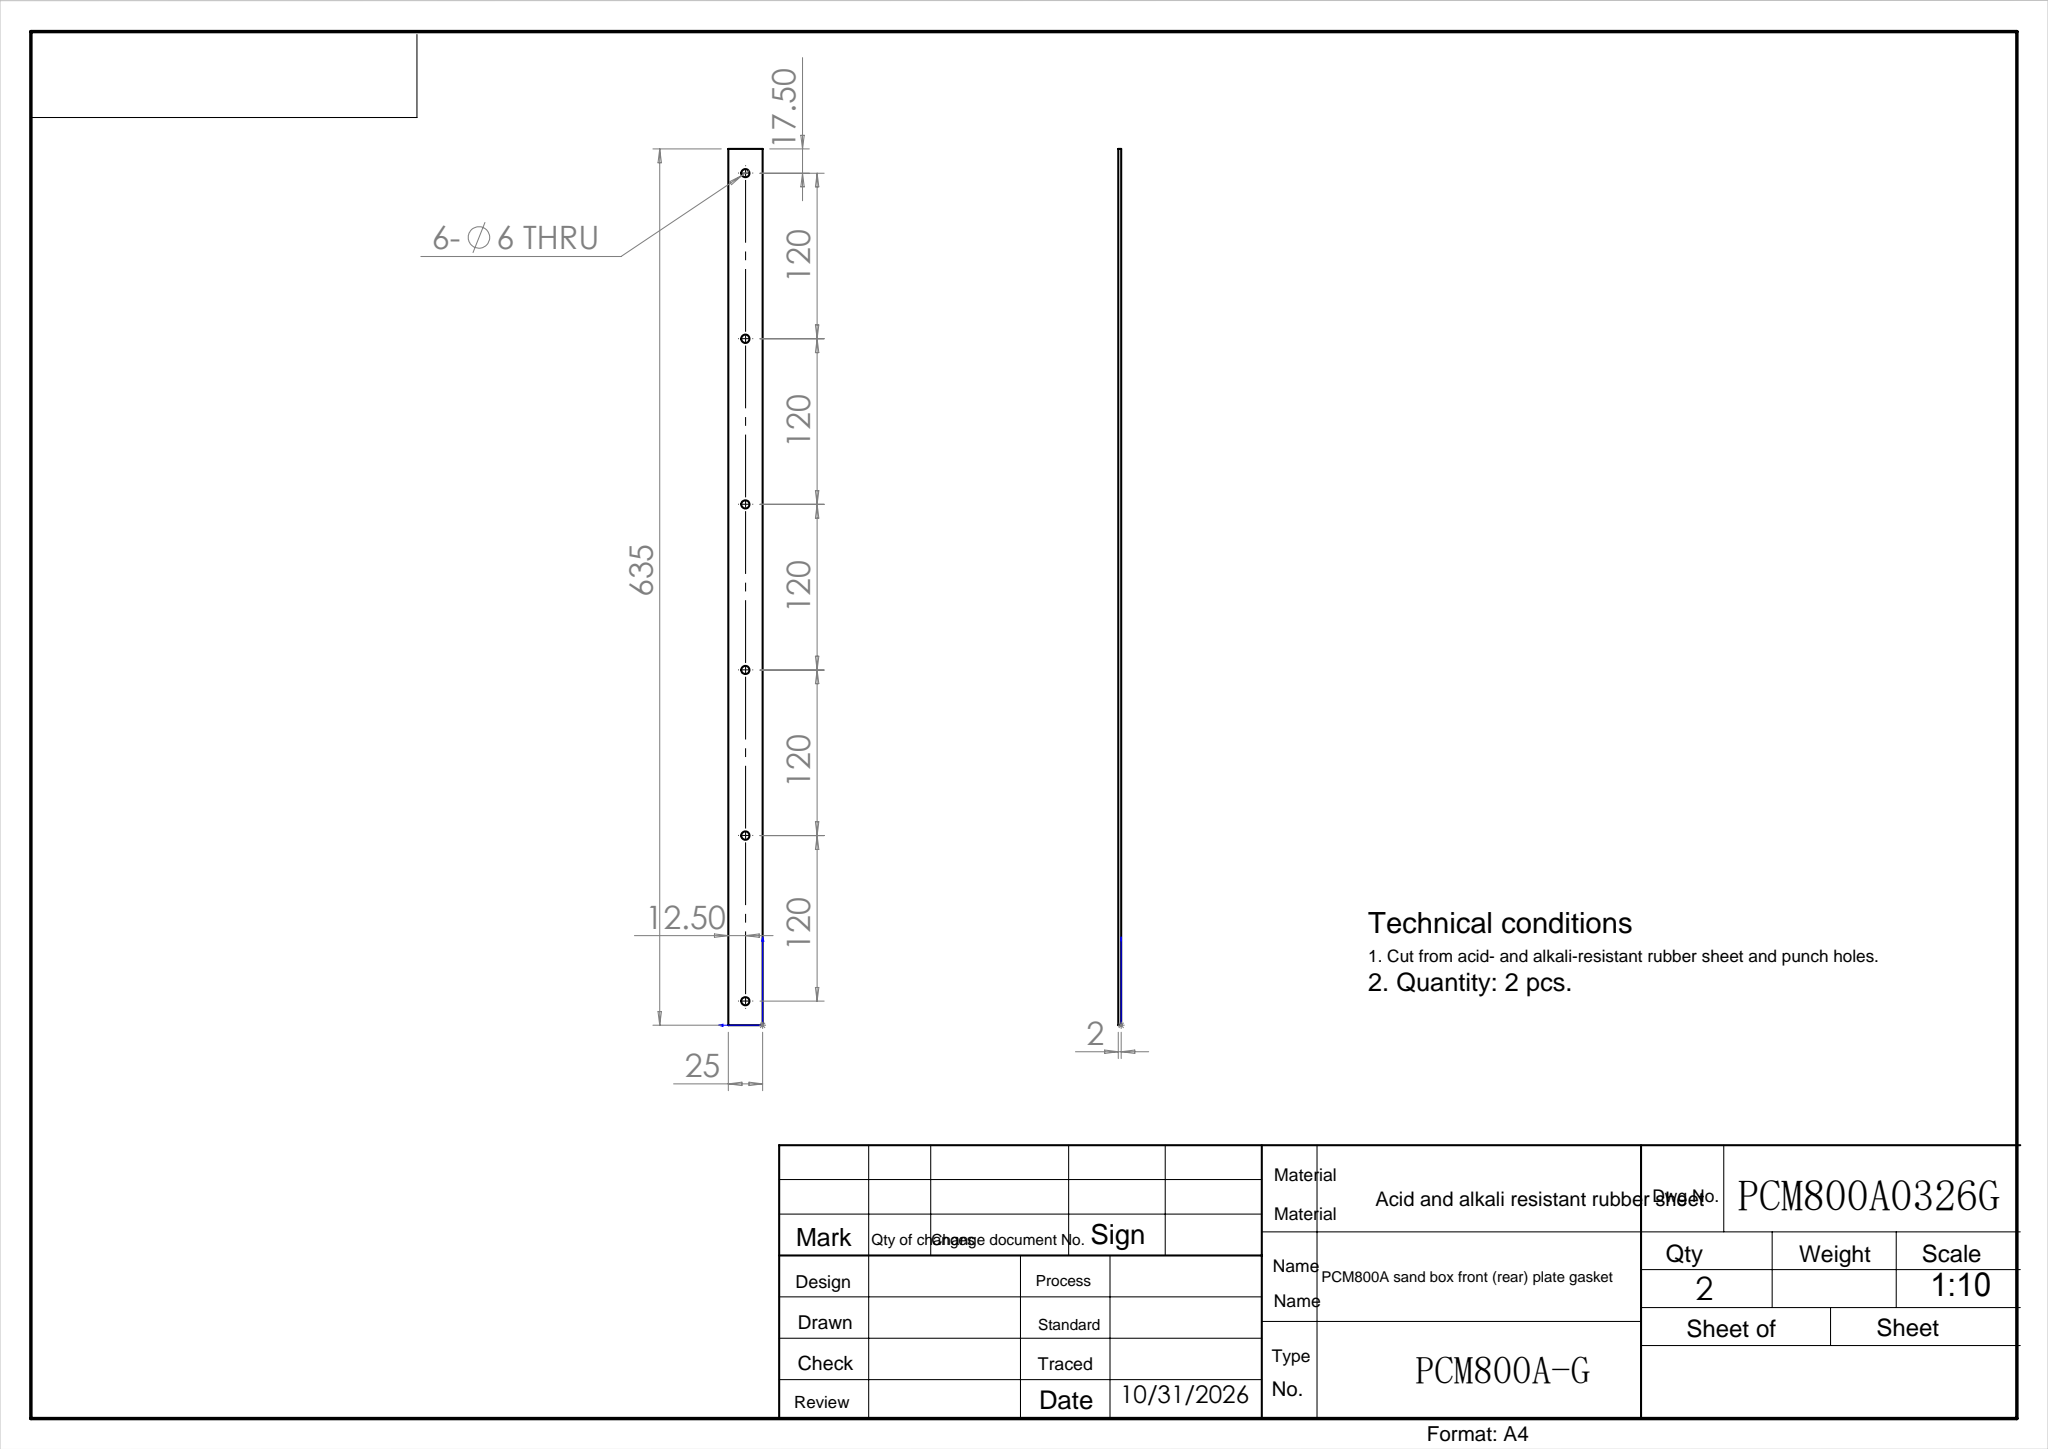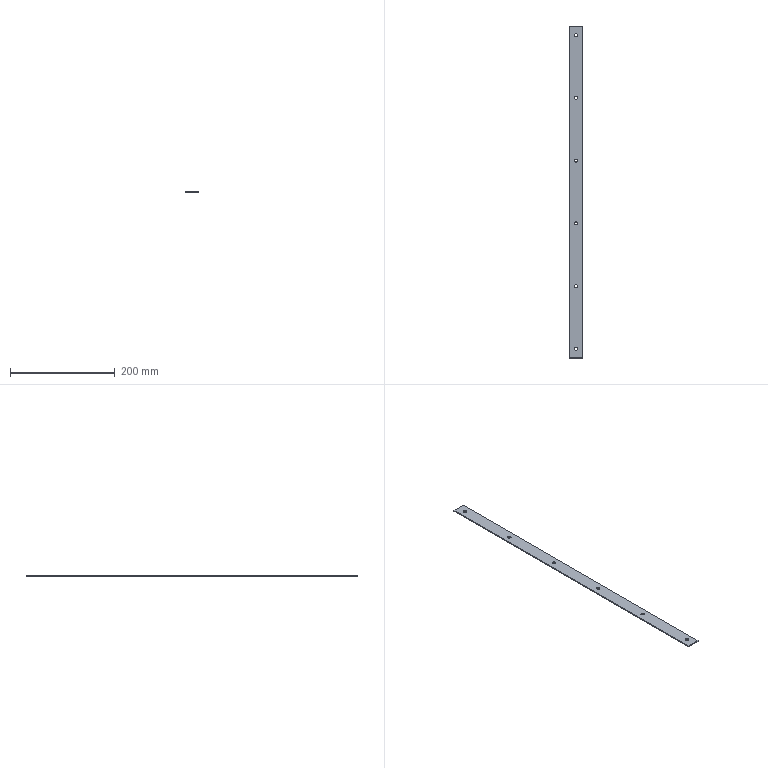Part | SolidWorks | features Cut 1, Extrusion 1, LPattern 1 | 1 solid | 18 faces | box 25 x 635 x 2 mm | volume 31411 mm3 | cylinder 12 | plane 6 | commonest cylinder face diameters 6 x12
STEP:
#1=CARTESIAN_POINT('',(9.5,17.5,0.));
#2=VERTEX_POINT('',#1);
#3=CARTESIAN_POINT('',(15.5,17.5,0.));
#4=VERTEX_POINT('',#3);
#5=CARTESIAN_POINT('',(12.5,17.5,0.));
#6=DIRECTION('',(0.,0.,1.));
#7=DIRECTION('',(1.,0.,0.));
#8=AXIS2_PLACEMENT_3D('',#5,#6,#7);
#9=CIRCLE('',#8,3.);
#10=EDGE_CURVE('',#2,#4,#9,.T.);
#11=ORIENTED_EDGE('',*,*,#10,.F.);
#12=CARTESIAN_POINT('',(9.5,17.5,2.));
#13=VERTEX_POINT('',#12);
#14=CARTESIAN_POINT('',(9.5,17.5,0.));
#15=DIRECTION('',(0.,0.,1.));
#16=VECTOR('',#15,1000.);
#17=LINE('',#14,#16);
#18=EDGE_CURVE('',#2,#13,#17,.T.);
#19=ORIENTED_EDGE('',*,*,#18,.T.);
#20=CARTESIAN_POINT('',(15.5,17.5,2.));
#21=VERTEX_POINT('',#20);
#22=CARTESIAN_POINT('',(12.5,17.5,2.));
#23=DIRECTION('',(0.,0.,1.));
#24=DIRECTION('',(1.,0.,0.));
#25=AXIS2_PLACEMENT_3D('',#22,#23,#24);
#26=CIRCLE('',#25,3.);
#27=EDGE_CURVE('',#13,#21,#26,.T.);
#28=ORIENTED_EDGE('',*,*,#27,.T.);
#29=CARTESIAN_POINT('',(15.5,17.5,0.));
#30=DIRECTION('',(0.,0.,1.));
#31=VECTOR('',#30,1000.);
#32=LINE('',#29,#31);
#33=EDGE_CURVE('',#4,#21,#32,.T.);
#34=ORIENTED_EDGE('',*,*,#33,.F.);
#35=EDGE_LOOP('',(#11,#19,#28,#34));
#36=FACE_OUTER_BOUND('',#35,.T.);
#37=CARTESIAN_POINT('',(12.5,17.5,0.));
#38=DIRECTION('',(0.,0.,1.));
#39=DIRECTION('',(1.,0.,0.));
#40=AXIS2_PLACEMENT_3D('',#37,#38,#39);
#41=CYLINDRICAL_SURFACE('',#40,3.);
#42=ADVANCED_FACE('',(#36),#41,.F.);
#43=CARTESIAN_POINT('',(9.5,137.5,0.));
#44=VERTEX_POINT('',#43);
#45=CARTESIAN_POINT('',(15.5,137.5,0.));
#46=VERTEX_POINT('',#45);
#47=CARTESIAN_POINT('',(12.5,137.5,0.));
#48=DIRECTION('',(0.,0.,1.));
#49=DIRECTION('',(1.,0.,0.));
#50=AXIS2_PLACEMENT_3D('',#47,#48,#49);
#51=CIRCLE('',#50,3.);
#52=EDGE_CURVE('',#44,#46,#51,.T.);
#53=ORIENTED_EDGE('',*,*,#52,.F.);
#54=CARTESIAN_POINT('',(9.5,137.5,2.));
#55=VERTEX_POINT('',#54);
#56=CARTESIAN_POINT('',(9.5,137.5,0.));
#57=DIRECTION('',(0.,0.,1.));
#58=VECTOR('',#57,1000.);
#59=LINE('',#56,#58);
#60=EDGE_CURVE('',#44,#55,#59,.T.);
#61=ORIENTED_EDGE('',*,*,#60,.T.);
#62=CARTESIAN_POINT('',(15.5,137.5,2.));
#63=VERTEX_POINT('',#62);
#64=CARTESIAN_POINT('',(12.5,137.5,2.));
#65=DIRECTION('',(0.,0.,1.));
#66=DIRECTION('',(1.,0.,0.));
#67=AXIS2_PLACEMENT_3D('',#64,#65,#66);
#68=CIRCLE('',#67,3.);
#69=EDGE_CURVE('',#55,#63,#68,.T.);
#70=ORIENTED_EDGE('',*,*,#69,.T.);
#71=CARTESIAN_POINT('',(15.5,137.5,0.));
#72=DIRECTION('',(0.,0.,1.));
#73=VECTOR('',#72,1000.);
#74=LINE('',#71,#73);
#75=EDGE_CURVE('',#46,#63,#74,.T.);
#76=ORIENTED_EDGE('',*,*,#75,.F.);
#77=EDGE_LOOP('',(#53,#61,#70,#76));
#78=FACE_OUTER_BOUND('',#77,.T.);
#79=CARTESIAN_POINT('',(12.5,137.5,0.));
#80=DIRECTION('',(0.,0.,1.));
#81=DIRECTION('',(1.,0.,0.));
#82=AXIS2_PLACEMENT_3D('',#79,#80,#81);
#83=CYLINDRICAL_SURFACE('',#82,3.);
#84=ADVANCED_FACE('',(#78),#83,.F.);
#85=CARTESIAN_POINT('',(9.5,257.5,0.));
#86=VERTEX_POINT('',#85);
#87=CARTESIAN_POINT('',(15.5,257.5,0.));
#88=VERTEX_POINT('',#87);
#89=CARTESIAN_POINT('',(12.5,257.5,0.));
#90=DIRECTION('',(0.,0.,1.));
#91=DIRECTION('',(1.,0.,0.));
#92=AXIS2_PLACEMENT_3D('',#89,#90,#91);
#93=CIRCLE('',#92,3.);
#94=EDGE_CURVE('',#86,#88,#93,.T.);
#95=ORIENTED_EDGE('',*,*,#94,.F.);
#96=CARTESIAN_POINT('',(9.5,257.5,2.));
#97=VERTEX_POINT('',#96);
#98=CARTESIAN_POINT('',(9.5,257.5,0.));
#99=DIRECTION('',(0.,0.,1.));
#100=VECTOR('',#99,1000.);
#101=LINE('',#98,#100);
#102=EDGE_CURVE('',#86,#97,#101,.T.);
#103=ORIENTED_EDGE('',*,*,#102,.T.);
#104=CARTESIAN_POINT('',(15.5,257.5,2.));
#105=VERTEX_POINT('',#104);
#106=CARTESIAN_POINT('',(12.5,257.5,2.));
#107=DIRECTION('',(0.,0.,1.));
#108=DIRECTION('',(1.,0.,0.));
#109=AXIS2_PLACEMENT_3D('',#106,#107,#108);
#110=CIRCLE('',#109,3.);
#111=EDGE_CURVE('',#97,#105,#110,.T.);
#112=ORIENTED_EDGE('',*,*,#111,.T.);
#113=CARTESIAN_POINT('',(15.5,257.5,0.));
#114=DIRECTION('',(0.,0.,1.));
#115=VECTOR('',#114,1000.);
#116=LINE('',#113,#115);
#117=EDGE_CURVE('',#88,#105,#116,.T.);
#118=ORIENTED_EDGE('',*,*,#117,.F.);
#119=EDGE_LOOP('',(#95,#103,#112,#118));
#120=FACE_OUTER_BOUND('',#119,.T.);
#121=CARTESIAN_POINT('',(12.5,257.5,0.));
#122=DIRECTION('',(0.,0.,1.));
#123=DIRECTION('',(1.,0.,0.));
#124=AXIS2_PLACEMENT_3D('',#121,#122,#123);
#125=CYLINDRICAL_SURFACE('',#124,3.);
#126=ADVANCED_FACE('',(#120),#125,.F.);
#127=CARTESIAN_POINT('',(9.5,377.5,0.));
#128=VERTEX_POINT('',#127);
#129=CARTESIAN_POINT('',(15.5,377.5,0.));
#130=VERTEX_POINT('',#129);
#131=CARTESIAN_POINT('',(12.5,377.5,0.));
#132=DIRECTION('',(0.,0.,1.));
#133=DIRECTION('',(1.,0.,0.));
#134=AXIS2_PLACEMENT_3D('',#131,#132,#133);
#135=CIRCLE('',#134,3.);
#136=EDGE_CURVE('',#128,#130,#135,.T.);
#137=ORIENTED_EDGE('',*,*,#136,.F.);
#138=CARTESIAN_POINT('',(9.5,377.5,2.));
#139=VERTEX_POINT('',#138);
#140=CARTESIAN_POINT('',(9.5,377.5,0.));
#141=DIRECTION('',(0.,0.,1.));
#142=VECTOR('',#141,1000.);
#143=LINE('',#140,#142);
#144=EDGE_CURVE('',#128,#139,#143,.T.);
#145=ORIENTED_EDGE('',*,*,#144,.T.);
#146=CARTESIAN_POINT('',(15.5,377.5,2.));
#147=VERTEX_POINT('',#146);
#148=CARTESIAN_POINT('',(12.5,377.5,2.));
#149=DIRECTION('',(0.,0.,1.));
#150=DIRECTION('',(1.,0.,0.));
#151=AXIS2_PLACEMENT_3D('',#148,#149,#150);
#152=CIRCLE('',#151,3.);
#153=EDGE_CURVE('',#139,#147,#152,.T.);
#154=ORIENTED_EDGE('',*,*,#153,.T.);
#155=CARTESIAN_POINT('',(15.5,377.5,0.));
#156=DIRECTION('',(0.,0.,1.));
#157=VECTOR('',#156,1000.);
#158=LINE('',#155,#157);
#159=EDGE_CURVE('',#130,#147,#158,.T.);
#160=ORIENTED_EDGE('',*,*,#159,.F.);
#161=EDGE_LOOP('',(#137,#145,#154,#160));
#162=FACE_OUTER_BOUND('',#161,.T.);
#163=CARTESIAN_POINT('',(12.5,377.5,0.));
#164=DIRECTION('',(0.,0.,1.));
#165=DIRECTION('',(1.,0.,0.));
#166=AXIS2_PLACEMENT_3D('',#163,#164,#165);
#167=CYLINDRICAL_SURFACE('',#166,3.);
#168=ADVANCED_FACE('',(#162),#167,.F.);
#169=CARTESIAN_POINT('',(9.5,497.5,0.));
#170=VERTEX_POINT('',#169);
#171=CARTESIAN_POINT('',(15.5,497.5,0.));
#172=VERTEX_POINT('',#171);
#173=CARTESIAN_POINT('',(12.5,497.5,0.));
#174=DIRECTION('',(0.,0.,1.));
#175=DIRECTION('',(1.,0.,0.));
#176=AXIS2_PLACEMENT_3D('',#173,#174,#175);
#177=CIRCLE('',#176,3.);
#178=EDGE_CURVE('',#170,#172,#177,.T.);
#179=ORIENTED_EDGE('',*,*,#178,.F.);
#180=CARTESIAN_POINT('',(9.5,497.5,2.));
#181=VERTEX_POINT('',#180);
#182=CARTESIAN_POINT('',(9.5,497.5,0.));
#183=DIRECTION('',(0.,0.,1.));
#184=VECTOR('',#183,1000.);
#185=LINE('',#182,#184);
#186=EDGE_CURVE('',#170,#181,#185,.T.);
#187=ORIENTED_EDGE('',*,*,#186,.T.);
#188=CARTESIAN_POINT('',(15.5,497.5,2.));
#189=VERTEX_POINT('',#188);
#190=CARTESIAN_POINT('',(12.5,497.5,2.));
#191=DIRECTION('',(0.,0.,1.));
#192=DIRECTION('',(1.,0.,0.));
#193=AXIS2_PLACEMENT_3D('',#190,#191,#192);
#194=CIRCLE('',#193,3.);
#195=EDGE_CURVE('',#181,#189,#194,.T.);
#196=ORIENTED_EDGE('',*,*,#195,.T.);
#197=CARTESIAN_POINT('',(15.5,497.5,0.));
#198=DIRECTION('',(0.,0.,1.));
#199=VECTOR('',#198,1000.);
#200=LINE('',#197,#199);
#201=EDGE_CURVE('',#172,#189,#200,.T.);
#202=ORIENTED_EDGE('',*,*,#201,.F.);
#203=EDGE_LOOP('',(#179,#187,#196,#202));
#204=FACE_OUTER_BOUND('',#203,.T.);
#205=CARTESIAN_POINT('',(12.5,497.5,0.));
#206=DIRECTION('',(0.,0.,1.));
#207=DIRECTION('',(1.,0.,0.));
#208=AXIS2_PLACEMENT_3D('',#205,#206,#207);
#209=CYLINDRICAL_SURFACE('',#208,3.);
#210=ADVANCED_FACE('',(#204),#209,.F.);
#211=CARTESIAN_POINT('',(9.5,617.5,0.));
#212=VERTEX_POINT('',#211);
#213=CARTESIAN_POINT('',(15.5,617.5,0.));
#214=VERTEX_POINT('',#213);
#215=CARTESIAN_POINT('',(12.5,617.5,0.));
#216=DIRECTION('',(0.,0.,1.));
#217=DIRECTION('',(1.,0.,0.));
#218=AXIS2_PLACEMENT_3D('',#215,#216,#217);
#219=CIRCLE('',#218,3.);
#220=EDGE_CURVE('',#212,#214,#219,.T.);
#221=ORIENTED_EDGE('',*,*,#220,.F.);
#222=CARTESIAN_POINT('',(9.5,617.5,2.));
#223=VERTEX_POINT('',#222);
#224=CARTESIAN_POINT('',(9.5,617.5,0.));
#225=DIRECTION('',(0.,0.,1.));
#226=VECTOR('',#225,1000.);
#227=LINE('',#224,#226);
#228=EDGE_CURVE('',#212,#223,#227,.T.);
#229=ORIENTED_EDGE('',*,*,#228,.T.);
#230=CARTESIAN_POINT('',(15.5,617.5,2.));
#231=VERTEX_POINT('',#230);
#232=CARTESIAN_POINT('',(12.5,617.5,2.));
#233=DIRECTION('',(0.,0.,1.));
#234=DIRECTION('',(1.,0.,0.));
#235=AXIS2_PLACEMENT_3D('',#232,#233,#234);
#236=CIRCLE('',#235,3.);
#237=EDGE_CURVE('',#223,#231,#236,.T.);
#238=ORIENTED_EDGE('',*,*,#237,.T.);
#239=CARTESIAN_POINT('',(15.5,617.5,0.));
#240=DIRECTION('',(0.,0.,1.));
#241=VECTOR('',#240,1000.);
#242=LINE('',#239,#241);
#243=EDGE_CURVE('',#214,#231,#242,.T.);
#244=ORIENTED_EDGE('',*,*,#243,.F.);
#245=EDGE_LOOP('',(#221,#229,#238,#244));
#246=FACE_OUTER_BOUND('',#245,.T.);
#247=CARTESIAN_POINT('',(12.5,617.5,0.));
#248=DIRECTION('',(0.,0.,1.));
#249=DIRECTION('',(1.,0.,0.));
#250=AXIS2_PLACEMENT_3D('',#247,#248,#249);
#251=CYLINDRICAL_SURFACE('',#250,3.);
#252=ADVANCED_FACE('',(#246),#251,.F.);
#253=CARTESIAN_POINT('',(0.,635.,0.));
#254=VERTEX_POINT('',#253);
#255=CARTESIAN_POINT('',(0.,0.,0.));
#256=VERTEX_POINT('',#255);
#257=CARTESIAN_POINT('',(0.,0.,0.));
#258=DIRECTION('',(0.,-1.,0.));
#259=VECTOR('',#258,1000.);
#260=LINE('',#257,#259);
#261=EDGE_CURVE('',#254,#256,#260,.T.);
#262=ORIENTED_EDGE('',*,*,#261,.T.);
#263=CARTESIAN_POINT('',(0.,0.,2.));
#264=VERTEX_POINT('',#263);
#265=CARTESIAN_POINT('',(0.,0.,2.));
#266=DIRECTION('',(0.,0.,-1.));
#267=VECTOR('',#266,1000.);
#268=LINE('',#265,#267);
#269=EDGE_CURVE('',#264,#256,#268,.T.);
#270=ORIENTED_EDGE('',*,*,#269,.F.);
#271=CARTESIAN_POINT('',(0.,635.,2.));
#272=VERTEX_POINT('',#271);
#273=CARTESIAN_POINT('',(0.,0.,2.));
#274=DIRECTION('',(0.,-1.,0.));
#275=VECTOR('',#274,1000.);
#276=LINE('',#273,#275);
#277=EDGE_CURVE('',#272,#264,#276,.T.);
#278=ORIENTED_EDGE('',*,*,#277,.F.);
#279=CARTESIAN_POINT('',(0.,635.,2.));
#280=DIRECTION('',(0.,0.,-1.));
#281=VECTOR('',#280,1000.);
#282=LINE('',#279,#281);
#283=EDGE_CURVE('',#272,#254,#282,.T.);
#284=ORIENTED_EDGE('',*,*,#283,.T.);
#285=EDGE_LOOP('',(#262,#270,#278,#284));
#286=FACE_OUTER_BOUND('',#285,.T.);
#287=CARTESIAN_POINT('',(0.,0.,2.));
#288=DIRECTION('',(1.,0.,0.));
#289=DIRECTION('',(0.,0.,-1.));
#290=AXIS2_PLACEMENT_3D('',#287,#288,#289);
#291=PLANE('',#290);
#292=ADVANCED_FACE('',(#286),#291,.F.);
#293=CARTESIAN_POINT('',(25.,0.,0.));
#294=VERTEX_POINT('',#293);
#295=CARTESIAN_POINT('',(0.,0.,0.));
#296=DIRECTION('',(1.,0.,0.));
#297=VECTOR('',#296,1000.);
#298=LINE('',#295,#297);
#299=EDGE_CURVE('',#256,#294,#298,.T.);
#300=ORIENTED_EDGE('',*,*,#299,.T.);
#301=CARTESIAN_POINT('',(25.,0.,2.));
#302=VERTEX_POINT('',#301);
#303=CARTESIAN_POINT('',(25.,0.,2.));
#304=DIRECTION('',(0.,0.,-1.));
#305=VECTOR('',#304,1000.);
#306=LINE('',#303,#305);
#307=EDGE_CURVE('',#302,#294,#306,.T.);
#308=ORIENTED_EDGE('',*,*,#307,.F.);
#309=CARTESIAN_POINT('',(0.,0.,2.));
#310=DIRECTION('',(1.,0.,0.));
#311=VECTOR('',#310,1000.);
#312=LINE('',#309,#311);
#313=EDGE_CURVE('',#264,#302,#312,.T.);
#314=ORIENTED_EDGE('',*,*,#313,.F.);
#315=ORIENTED_EDGE('',*,*,#269,.T.);
#316=EDGE_LOOP('',(#300,#308,#314,#315));
#317=FACE_OUTER_BOUND('',#316,.T.);
#318=CARTESIAN_POINT('',(0.,0.,2.));
#319=DIRECTION('',(0.,1.,0.));
#320=DIRECTION('',(0.,0.,1.));
#321=AXIS2_PLACEMENT_3D('',#318,#319,#320);
#322=PLANE('',#321);
#323=ADVANCED_FACE('',(#317),#322,.F.);
#324=CARTESIAN_POINT('',(25.,635.,0.));
#325=VERTEX_POINT('',#324);
#326=CARTESIAN_POINT('',(25.,0.,0.));
#327=DIRECTION('',(0.,1.,0.));
#328=VECTOR('',#327,1000.);
#329=LINE('',#326,#328);
#330=EDGE_CURVE('',#294,#325,#329,.T.);
#331=ORIENTED_EDGE('',*,*,#330,.T.);
#332=CARTESIAN_POINT('',(25.,635.,2.));
#333=VERTEX_POINT('',#332);
#334=CARTESIAN_POINT('',(25.,635.,2.));
#335=DIRECTION('',(0.,0.,-1.));
#336=VECTOR('',#335,1000.);
#337=LINE('',#334,#336);
#338=EDGE_CURVE('',#333,#325,#337,.T.);
#339=ORIENTED_EDGE('',*,*,#338,.F.);
#340=CARTESIAN_POINT('',(25.,0.,2.));
#341=DIRECTION('',(0.,1.,0.));
#342=VECTOR('',#341,1000.);
#343=LINE('',#340,#342);
#344=EDGE_CURVE('',#302,#333,#343,.T.);
#345=ORIENTED_EDGE('',*,*,#344,.F.);
#346=ORIENTED_EDGE('',*,*,#307,.T.);
#347=EDGE_LOOP('',(#331,#339,#345,#346));
#348=FACE_OUTER_BOUND('',#347,.T.);
#349=CARTESIAN_POINT('',(25.,0.,2.));
#350=DIRECTION('',(-1.,0.,0.));
#351=DIRECTION('',(0.,0.,1.));
#352=AXIS2_PLACEMENT_3D('',#349,#350,#351);
#353=PLANE('',#352);
#354=ADVANCED_FACE('',(#348),#353,.F.);
#355=CARTESIAN_POINT('',(0.,635.,0.));
#356=DIRECTION('',(-1.,0.,0.));
#357=VECTOR('',#356,1000.);
#358=LINE('',#355,#357);
#359=EDGE_CURVE('',#325,#254,#358,.T.);
#360=ORIENTED_EDGE('',*,*,#359,.T.);
#361=ORIENTED_EDGE('',*,*,#283,.F.);
#362=CARTESIAN_POINT('',(0.,635.,2.));
#363=DIRECTION('',(-1.,0.,0.));
#364=VECTOR('',#363,1000.);
#365=LINE('',#362,#364);
#366=EDGE_CURVE('',#333,#272,#365,.T.);
#367=ORIENTED_EDGE('',*,*,#366,.F.);
#368=ORIENTED_EDGE('',*,*,#338,.T.);
#369=EDGE_LOOP('',(#360,#361,#367,#368));
#370=FACE_OUTER_BOUND('',#369,.T.);
#371=CARTESIAN_POINT('',(0.,635.,2.));
#372=DIRECTION('',(0.,-1.,0.));
#373=DIRECTION('',(0.,0.,-1.));
#374=AXIS2_PLACEMENT_3D('',#371,#372,#373);
#375=PLANE('',#374);
#376=ADVANCED_FACE('',(#370),#375,.F.);
#377=CARTESIAN_POINT('',(12.5,17.5,2.));
#378=DIRECTION('',(0.,0.,1.));
#379=DIRECTION('',(1.,0.,0.));
#380=AXIS2_PLACEMENT_3D('',#377,#378,#379);
#381=CIRCLE('',#380,3.);
#382=EDGE_CURVE('',#21,#13,#381,.T.);
#383=ORIENTED_EDGE('',*,*,#382,.F.);
#384=ORIENTED_EDGE('',*,*,#27,.F.);
#385=EDGE_LOOP('',(#383,#384));
#386=FACE_BOUND('',#385,.T.);
#387=CARTESIAN_POINT('',(12.5,137.5,2.));
#388=DIRECTION('',(0.,0.,1.));
#389=DIRECTION('',(1.,0.,0.));
#390=AXIS2_PLACEMENT_3D('',#387,#388,#389);
#391=CIRCLE('',#390,3.);
#392=EDGE_CURVE('',#63,#55,#391,.T.);
#393=ORIENTED_EDGE('',*,*,#392,.F.);
#394=ORIENTED_EDGE('',*,*,#69,.F.);
#395=EDGE_LOOP('',(#393,#394));
#396=FACE_BOUND('',#395,.T.);
#397=CARTESIAN_POINT('',(12.5,257.5,2.));
#398=DIRECTION('',(0.,0.,1.));
#399=DIRECTION('',(1.,0.,0.));
#400=AXIS2_PLACEMENT_3D('',#397,#398,#399);
#401=CIRCLE('',#400,3.);
#402=EDGE_CURVE('',#105,#97,#401,.T.);
#403=ORIENTED_EDGE('',*,*,#402,.F.);
#404=ORIENTED_EDGE('',*,*,#111,.F.);
#405=EDGE_LOOP('',(#403,#404));
#406=FACE_BOUND('',#405,.T.);
#407=CARTESIAN_POINT('',(12.5,377.5,2.));
#408=DIRECTION('',(0.,0.,1.));
#409=DIRECTION('',(1.,0.,0.));
#410=AXIS2_PLACEMENT_3D('',#407,#408,#409);
#411=CIRCLE('',#410,3.);
#412=EDGE_CURVE('',#147,#139,#411,.T.);
#413=ORIENTED_EDGE('',*,*,#412,.F.);
#414=ORIENTED_EDGE('',*,*,#153,.F.);
#415=EDGE_LOOP('',(#413,#414));
#416=FACE_BOUND('',#415,.T.);
#417=CARTESIAN_POINT('',(12.5,497.5,2.));
#418=DIRECTION('',(0.,0.,1.));
#419=DIRECTION('',(1.,0.,0.));
#420=AXIS2_PLACEMENT_3D('',#417,#418,#419);
#421=CIRCLE('',#420,3.);
#422=EDGE_CURVE('',#189,#181,#421,.T.);
#423=ORIENTED_EDGE('',*,*,#422,.F.);
#424=ORIENTED_EDGE('',*,*,#195,.F.);
#425=EDGE_LOOP('',(#423,#424));
#426=FACE_BOUND('',#425,.T.);
#427=CARTESIAN_POINT('',(12.5,617.5,2.));
#428=DIRECTION('',(0.,0.,1.));
#429=DIRECTION('',(1.,0.,0.));
#430=AXIS2_PLACEMENT_3D('',#427,#428,#429);
#431=CIRCLE('',#430,3.);
#432=EDGE_CURVE('',#231,#223,#431,.T.);
#433=ORIENTED_EDGE('',*,*,#432,.F.);
#434=ORIENTED_EDGE('',*,*,#237,.F.);
#435=EDGE_LOOP('',(#433,#434));
#436=FACE_BOUND('',#435,.T.);
#437=ORIENTED_EDGE('',*,*,#277,.T.);
#438=ORIENTED_EDGE('',*,*,#313,.T.);
#439=ORIENTED_EDGE('',*,*,#344,.T.);
#440=ORIENTED_EDGE('',*,*,#366,.T.);
#441=EDGE_LOOP('',(#437,#438,#439,#440));
#442=FACE_OUTER_BOUND('',#441,.T.);
#443=CARTESIAN_POINT('',(0.,635.,2.));
#444=DIRECTION('',(0.,0.,-1.));
#445=DIRECTION('',(-1.,0.,0.));
#446=AXIS2_PLACEMENT_3D('',#443,#444,#445);
#447=PLANE('',#446);
#448=ADVANCED_FACE('',(#386,#396,#406,#416,#426,#436,#442),#447,.F.);
#449=CARTESIAN_POINT('',(12.5,17.5,0.));
#450=DIRECTION('',(0.,0.,1.));
#451=DIRECTION('',(1.,0.,0.));
#452=AXIS2_PLACEMENT_3D('',#449,#450,#451);
#453=CIRCLE('',#452,3.);
#454=EDGE_CURVE('',#4,#2,#453,.T.);
#455=ORIENTED_EDGE('',*,*,#454,.T.);
#456=ORIENTED_EDGE('',*,*,#10,.T.);
#457=EDGE_LOOP('',(#455,#456));
#458=FACE_BOUND('',#457,.T.);
#459=CARTESIAN_POINT('',(12.5,137.5,0.));
#460=DIRECTION('',(0.,0.,1.));
#461=DIRECTION('',(1.,0.,0.));
#462=AXIS2_PLACEMENT_3D('',#459,#460,#461);
#463=CIRCLE('',#462,3.);
#464=EDGE_CURVE('',#46,#44,#463,.T.);
#465=ORIENTED_EDGE('',*,*,#464,.T.);
#466=ORIENTED_EDGE('',*,*,#52,.T.);
#467=EDGE_LOOP('',(#465,#466));
#468=FACE_BOUND('',#467,.T.);
#469=CARTESIAN_POINT('',(12.5,257.5,0.));
#470=DIRECTION('',(0.,0.,1.));
#471=DIRECTION('',(1.,0.,0.));
#472=AXIS2_PLACEMENT_3D('',#469,#470,#471);
#473=CIRCLE('',#472,3.);
#474=EDGE_CURVE('',#88,#86,#473,.T.);
#475=ORIENTED_EDGE('',*,*,#474,.T.);
#476=ORIENTED_EDGE('',*,*,#94,.T.);
#477=EDGE_LOOP('',(#475,#476));
#478=FACE_BOUND('',#477,.T.);
#479=CARTESIAN_POINT('',(12.5,377.5,0.));
#480=DIRECTION('',(0.,0.,1.));
#481=DIRECTION('',(1.,0.,0.));
#482=AXIS2_PLACEMENT_3D('',#479,#480,#481);
#483=CIRCLE('',#482,3.);
#484=EDGE_CURVE('',#130,#128,#483,.T.);
#485=ORIENTED_EDGE('',*,*,#484,.T.);
#486=ORIENTED_EDGE('',*,*,#136,.T.);
#487=EDGE_LOOP('',(#485,#486));
#488=FACE_BOUND('',#487,.T.);
#489=CARTESIAN_POINT('',(12.5,497.5,0.));
#490=DIRECTION('',(0.,0.,1.));
#491=DIRECTION('',(1.,0.,0.));
#492=AXIS2_PLACEMENT_3D('',#489,#490,#491);
#493=CIRCLE('',#492,3.);
#494=EDGE_CURVE('',#172,#170,#493,.T.);
#495=ORIENTED_EDGE('',*,*,#494,.T.);
#496=ORIENTED_EDGE('',*,*,#178,.T.);
#497=EDGE_LOOP('',(#495,#496));
#498=FACE_BOUND('',#497,.T.);
#499=CARTESIAN_POINT('',(12.5,617.5,0.));
#500=DIRECTION('',(0.,0.,1.));
#501=DIRECTION('',(1.,0.,0.));
#502=AXIS2_PLACEMENT_3D('',#499,#500,#501);
#503=CIRCLE('',#502,3.);
#504=EDGE_CURVE('',#214,#212,#503,.T.);
#505=ORIENTED_EDGE('',*,*,#504,.T.);
#506=ORIENTED_EDGE('',*,*,#220,.T.);
#507=EDGE_LOOP('',(#505,#506));
#508=FACE_BOUND('',#507,.T.);
#509=ORIENTED_EDGE('',*,*,#261,.F.);
#510=ORIENTED_EDGE('',*,*,#359,.F.);
#511=ORIENTED_EDGE('',*,*,#330,.F.);
#512=ORIENTED_EDGE('',*,*,#299,.F.);
#513=EDGE_LOOP('',(#509,#510,#511,#512));
#514=FACE_OUTER_BOUND('',#513,.T.);
#515=CARTESIAN_POINT('',(0.,635.,0.));
#516=DIRECTION('',(0.,0.,-1.));
#517=DIRECTION('',(-1.,0.,0.));
#518=AXIS2_PLACEMENT_3D('',#515,#516,#517);
#519=PLANE('',#518);
#520=ADVANCED_FACE('',(#458,#468,#478,#488,#498,#508,#514),#519,.T.);
#521=ORIENTED_EDGE('',*,*,#228,.F.);
#522=ORIENTED_EDGE('',*,*,#504,.F.);
#523=ORIENTED_EDGE('',*,*,#243,.T.);
#524=ORIENTED_EDGE('',*,*,#432,.T.);
#525=EDGE_LOOP('',(#521,#522,#523,#524));
#526=FACE_OUTER_BOUND('',#525,.T.);
#527=CARTESIAN_POINT('',(12.5,617.5,0.));
#528=DIRECTION('',(0.,0.,1.));
#529=DIRECTION('',(1.,0.,0.));
#530=AXIS2_PLACEMENT_3D('',#527,#528,#529);
#531=CYLINDRICAL_SURFACE('',#530,3.);
#532=ADVANCED_FACE('',(#526),#531,.F.);
#533=ORIENTED_EDGE('',*,*,#186,.F.);
#534=ORIENTED_EDGE('',*,*,#494,.F.);
#535=ORIENTED_EDGE('',*,*,#201,.T.);
#536=ORIENTED_EDGE('',*,*,#422,.T.);
#537=EDGE_LOOP('',(#533,#534,#535,#536));
#538=FACE_OUTER_BOUND('',#537,.T.);
#539=CARTESIAN_POINT('',(12.5,497.5,0.));
#540=DIRECTION('',(0.,0.,1.));
#541=DIRECTION('',(1.,0.,0.));
#542=AXIS2_PLACEMENT_3D('',#539,#540,#541);
#543=CYLINDRICAL_SURFACE('',#542,3.);
#544=ADVANCED_FACE('',(#538),#543,.F.);
#545=ORIENTED_EDGE('',*,*,#144,.F.);
#546=ORIENTED_EDGE('',*,*,#484,.F.);
#547=ORIENTED_EDGE('',*,*,#159,.T.);
#548=ORIENTED_EDGE('',*,*,#412,.T.);
#549=EDGE_LOOP('',(#545,#546,#547,#548));
#550=FACE_OUTER_BOUND('',#549,.T.);
#551=CARTESIAN_POINT('',(12.5,377.5,0.));
#552=DIRECTION('',(0.,0.,1.));
#553=DIRECTION('',(1.,0.,0.));
#554=AXIS2_PLACEMENT_3D('',#551,#552,#553);
#555=CYLINDRICAL_SURFACE('',#554,3.);
#556=ADVANCED_FACE('',(#550),#555,.F.);
#557=ORIENTED_EDGE('',*,*,#102,.F.);
#558=ORIENTED_EDGE('',*,*,#474,.F.);
#559=ORIENTED_EDGE('',*,*,#117,.T.);
#560=ORIENTED_EDGE('',*,*,#402,.T.);
#561=EDGE_LOOP('',(#557,#558,#559,#560));
#562=FACE_OUTER_BOUND('',#561,.T.);
#563=CARTESIAN_POINT('',(12.5,257.5,0.));
#564=DIRECTION('',(0.,0.,1.));
#565=DIRECTION('',(1.,0.,0.));
#566=AXIS2_PLACEMENT_3D('',#563,#564,#565);
#567=CYLINDRICAL_SURFACE('',#566,3.);
#568=ADVANCED_FACE('',(#562),#567,.F.);
#569=ORIENTED_EDGE('',*,*,#60,.F.);
#570=ORIENTED_EDGE('',*,*,#464,.F.);
#571=ORIENTED_EDGE('',*,*,#75,.T.);
#572=ORIENTED_EDGE('',*,*,#392,.T.);
#573=EDGE_LOOP('',(#569,#570,#571,#572));
#574=FACE_OUTER_BOUND('',#573,.T.);
#575=CARTESIAN_POINT('',(12.5,137.5,0.));
#576=DIRECTION('',(0.,0.,1.));
#577=DIRECTION('',(1.,0.,0.));
#578=AXIS2_PLACEMENT_3D('',#575,#576,#577);
#579=CYLINDRICAL_SURFACE('',#578,3.);
#580=ADVANCED_FACE('',(#574),#579,.F.);
#581=ORIENTED_EDGE('',*,*,#18,.F.);
#582=ORIENTED_EDGE('',*,*,#454,.F.);
#583=ORIENTED_EDGE('',*,*,#33,.T.);
#584=ORIENTED_EDGE('',*,*,#382,.T.);
#585=EDGE_LOOP('',(#581,#582,#583,#584));
#586=FACE_OUTER_BOUND('',#585,.T.);
#587=CARTESIAN_POINT('',(12.5,17.5,0.));
#588=DIRECTION('',(0.,0.,1.));
#589=DIRECTION('',(1.,0.,0.));
#590=AXIS2_PLACEMENT_3D('',#587,#588,#589);
#591=CYLINDRICAL_SURFACE('',#590,3.);
#592=ADVANCED_FACE('',(#586),#591,.F.);
#593=CLOSED_SHELL('',(#42,#84,#126,#168,#210,#252,#292,#323,#354,#376,#448,#520,#532,#544,#556,#568,#580,#592));
#594=MANIFOLD_SOLID_BREP('',#593);
#595=CARTESIAN_POINT('',(0.,0.,0.));
#596=DIRECTION('',(0.,0.,1.));
#597=DIRECTION('',(1.,0.,0.));
#598=AXIS2_PLACEMENT_3D('',#595,#596,#597);
#599=(LENGTH_UNIT()NAMED_UNIT(*)SI_UNIT(.MILLI.,.METRE.));
#600=UNCERTAINTY_MEASURE_WITH_UNIT(LENGTH_MEASURE(0.00001),#599,'','');
#601=(NAMED_UNIT(*)PLANE_ANGLE_UNIT()SI_UNIT($,.RADIAN.));
#602=(NAMED_UNIT(*)SI_UNIT($,.STERADIAN.)SOLID_ANGLE_UNIT());
#603=(GEOMETRIC_REPRESENTATION_CONTEXT(3)GLOBAL_UNCERTAINTY_ASSIGNED_CONTEXT((#600))GLOBAL_UNIT_ASSIGNED_CONTEXT((#599,#601,#602))REPRESENTATION_CONTEXT('',''));
#604=ADVANCED_BREP_SHAPE_REPRESENTATION('',(#594,#598),#603);